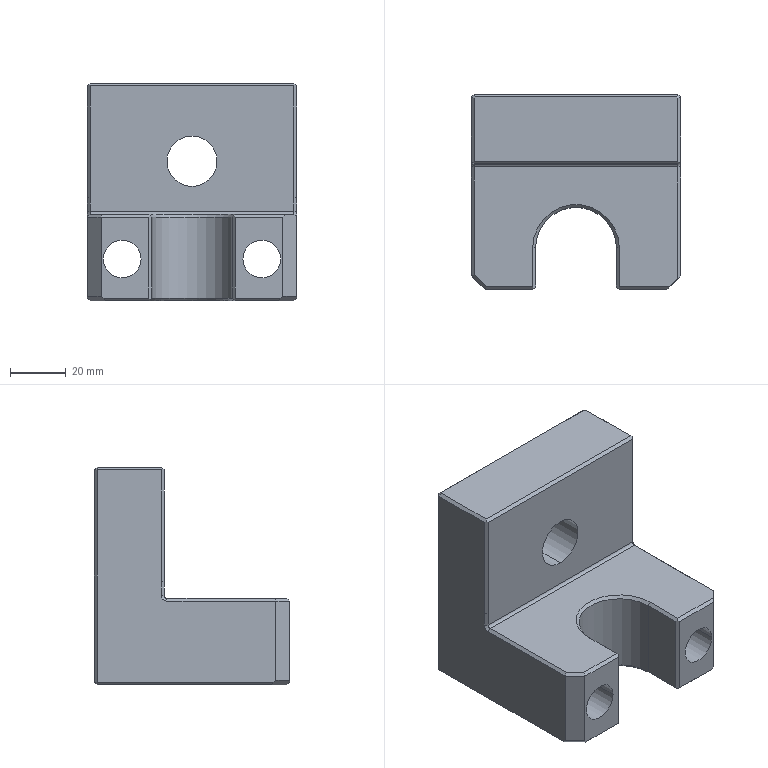Part | Creo | 1 solid | 90 faces | box 75 x 70 x 78 mm | volume 188512 mm3 | plane 48 | cylinder 26 | cone 16 | commonest cylinder face diameters 4.97 x6 6 x6 13.5 x4 20 x4 18 x2 41 x2